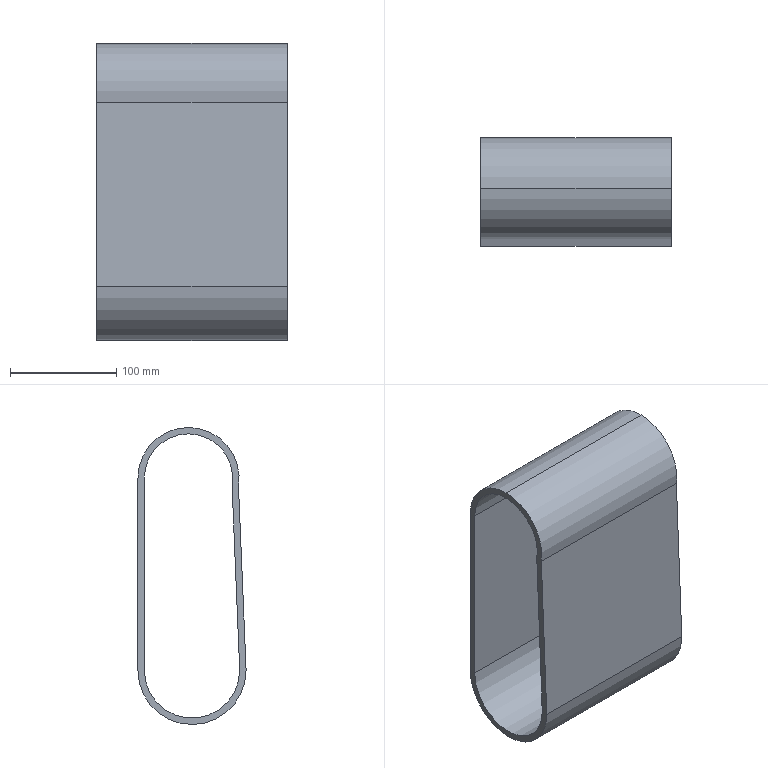Part | NX | 1 solid | 12 faces | box 180 x 102 x 280.001 mm | volume 706349 mm3 | cylinder 6 | plane 6 | commonest cylinder face diameters 83.424 x2 95.424 x2 90 x1 102 x1
STEP:
#1=CARTESIAN_POINT('',(220.674,202.789,606.798));
#2=VERTEX_POINT('',#1);
#3=CARTESIAN_POINT('',(220.674,244.501,565.086));
#4=VERTEX_POINT('',#3);
#5=CARTESIAN_POINT('',(220.674,202.789,565.086));
#6=DIRECTION('',(-1.,0.,0.));
#7=DIRECTION('',(0.,0.,1.));
#8=AXIS2_PLACEMENT_3D('',#5,#6,#7);
#9=CIRCLE('',#8,41.712);
#10=EDGE_CURVE('',#2,#4,#9,.T.);
#11=ORIENTED_EDGE('',*,*,#10,.F.);
#12=CARTESIAN_POINT('',(40.674,202.789,606.798));
#13=VERTEX_POINT('',#12);
#14=CARTESIAN_POINT('',(518.674,202.789,606.798));
#15=DIRECTION('',(-1.,0.,0.));
#16=VECTOR('',#15,1.);
#17=LINE('',#14,#16);
#18=EDGE_CURVE('',#2,#13,#17,.T.);
#19=ORIENTED_EDGE('',*,*,#18,.T.);
#20=CARTESIAN_POINT('',(40.674,244.501,565.086));
#21=VERTEX_POINT('',#20);
#22=CARTESIAN_POINT('',(40.674,202.789,565.086));
#23=DIRECTION('',(1.,0.,0.));
#24=DIRECTION('',(0.,0.,-1.));
#25=AXIS2_PLACEMENT_3D('',#22,#23,#24);
#26=CIRCLE('',#25,41.712);
#27=EDGE_CURVE('',#21,#13,#26,.T.);
#28=ORIENTED_EDGE('',*,*,#27,.F.);
#29=CARTESIAN_POINT('',(518.674,244.501,565.086));
#30=DIRECTION('',(-1.,0.,0.));
#31=VECTOR('',#30,1.);
#32=LINE('',#29,#31);
#33=EDGE_CURVE('',#4,#21,#32,.T.);
#34=ORIENTED_EDGE('',*,*,#33,.F.);
#35=EDGE_LOOP('',(#11,#19,#28,#34));
#36=FACE_OUTER_BOUND('',#35,.T.);
#37=CARTESIAN_POINT('',(518.674,202.789,565.086));
#38=DIRECTION('',(-1.,0.,0.));
#39=DIRECTION('',(0.,0.,1.));
#40=AXIS2_PLACEMENT_3D('',#37,#38,#39);
#41=CYLINDRICAL_SURFACE('',#40,41.712);
#42=ADVANCED_FACE('',(#36),#41,.F.);
#43=CARTESIAN_POINT('',(220.674,155.708,557.353));
#44=VERTEX_POINT('',#43);
#45=CARTESIAN_POINT('',(220.674,202.789,612.798));
#46=VERTEX_POINT('',#45);
#47=CARTESIAN_POINT('',(220.674,202.789,565.086));
#48=DIRECTION('',(-1.,0.,0.));
#49=DIRECTION('',(0.,0.,1.));
#50=AXIS2_PLACEMENT_3D('',#47,#48,#49);
#51=CIRCLE('',#50,47.712);
#52=EDGE_CURVE('',#44,#46,#51,.T.);
#53=ORIENTED_EDGE('',*,*,#52,.T.);
#54=CARTESIAN_POINT('',(40.674,202.789,612.798));
#55=VERTEX_POINT('',#54);
#56=CARTESIAN_POINT('',(518.674,202.789,612.798));
#57=DIRECTION('',(-1.,0.,0.));
#58=VECTOR('',#57,1.);
#59=LINE('',#56,#58);
#60=EDGE_CURVE('',#46,#55,#59,.T.);
#61=ORIENTED_EDGE('',*,*,#60,.T.);
#62=CARTESIAN_POINT('',(40.674,155.708,557.353));
#63=VERTEX_POINT('',#62);
#64=CARTESIAN_POINT('',(40.674,202.789,565.086));
#65=DIRECTION('',(1.,0.,0.));
#66=DIRECTION('',(0.,0.,-1.));
#67=AXIS2_PLACEMENT_3D('',#64,#65,#66);
#68=CIRCLE('',#67,47.712);
#69=EDGE_CURVE('',#55,#63,#68,.T.);
#70=ORIENTED_EDGE('',*,*,#69,.T.);
#71=CARTESIAN_POINT('',(518.674,155.708,557.353));
#72=DIRECTION('',(-1.,0.,0.));
#73=VECTOR('',#72,1.);
#74=LINE('',#71,#73);
#75=EDGE_CURVE('',#44,#63,#74,.T.);
#76=ORIENTED_EDGE('',*,*,#75,.F.);
#77=EDGE_LOOP('',(#53,#61,#70,#76));
#78=FACE_OUTER_BOUND('',#77,.T.);
#79=CARTESIAN_POINT('',(518.674,202.789,565.086));
#80=DIRECTION('',(-1.,0.,0.));
#81=DIRECTION('',(0.,0.,1.));
#82=AXIS2_PLACEMENT_3D('',#79,#80,#81);
#83=CYLINDRICAL_SURFACE('',#82,47.712);
#84=ADVANCED_FACE('',(#78),#83,.T.);
#85=CARTESIAN_POINT('',(40.674,148.501,383.926));
#86=VERTEX_POINT('',#85);
#87=CARTESIAN_POINT('',(40.674,250.501,383.798));
#88=VERTEX_POINT('',#87);
#89=CARTESIAN_POINT('',(40.674,199.501,383.798));
#90=DIRECTION('',(1.,0.,0.));
#91=DIRECTION('',(0.,0.,-1.));
#92=AXIS2_PLACEMENT_3D('',#89,#90,#91);
#93=CIRCLE('',#92,51.);
#94=EDGE_CURVE('',#86,#88,#93,.T.);
#95=ORIENTED_EDGE('',*,*,#94,.F.);
#96=CARTESIAN_POINT('',(40.674,148.506,384.047));
#97=DIRECTION('',(0.,-0.04152,-0.9991));
#98=VECTOR('',#97,1.);
#99=LINE('',#96,#98);
#100=EDGE_CURVE('',#63,#86,#99,.T.);
#101=ORIENTED_EDGE('',*,*,#100,.F.);
#102=ORIENTED_EDGE('',*,*,#69,.F.);
#103=CARTESIAN_POINT('',(40.674,250.501,565.086));
#104=VERTEX_POINT('',#103);
#105=CARTESIAN_POINT('',(40.674,202.789,565.086));
#106=DIRECTION('',(1.,0.,0.));
#107=DIRECTION('',(0.,0.,-1.));
#108=AXIS2_PLACEMENT_3D('',#105,#106,#107);
#109=CIRCLE('',#108,47.712);
#110=EDGE_CURVE('',#104,#55,#109,.T.);
#111=ORIENTED_EDGE('',*,*,#110,.F.);
#112=CARTESIAN_POINT('',(40.674,250.501,383.798));
#113=DIRECTION('',(0.,0.,1.));
#114=VECTOR('',#113,1.);
#115=LINE('',#112,#114);
#116=EDGE_CURVE('',#88,#104,#115,.T.);
#117=ORIENTED_EDGE('',*,*,#116,.F.);
#118=EDGE_LOOP('',(#95,#101,#102,#111,#117));
#119=FACE_BOUND('',#118,.T.);
#120=CARTESIAN_POINT('',(40.674,154.501,383.798));
#121=VERTEX_POINT('',#120);
#122=CARTESIAN_POINT('',(40.674,244.501,383.798));
#123=VERTEX_POINT('',#122);
#124=CARTESIAN_POINT('',(40.674,199.501,383.798));
#125=DIRECTION('',(1.,0.,0.));
#126=DIRECTION('',(0.,0.,-1.));
#127=AXIS2_PLACEMENT_3D('',#124,#125,#126);
#128=CIRCLE('',#127,45.);
#129=EDGE_CURVE('',#121,#123,#128,.T.);
#130=ORIENTED_EDGE('',*,*,#129,.T.);
#131=CARTESIAN_POINT('',(40.674,244.501,383.798));
#132=DIRECTION('',(0.,0.,1.));
#133=VECTOR('',#132,1.);
#134=LINE('',#131,#133);
#135=EDGE_CURVE('',#123,#21,#134,.T.);
#136=ORIENTED_EDGE('',*,*,#135,.T.);
#137=ORIENTED_EDGE('',*,*,#27,.T.);
#138=CARTESIAN_POINT('',(40.674,161.729,557.739));
#139=VERTEX_POINT('',#138);
#140=CARTESIAN_POINT('',(40.674,202.789,565.086));
#141=DIRECTION('',(1.,0.,0.));
#142=DIRECTION('',(0.,0.,-1.));
#143=AXIS2_PLACEMENT_3D('',#140,#141,#142);
#144=CIRCLE('',#143,41.712);
#145=EDGE_CURVE('',#13,#139,#144,.T.);
#146=ORIENTED_EDGE('',*,*,#145,.T.);
#147=CARTESIAN_POINT('',(40.674,154.501,383.798));
#148=DIRECTION('',(0.,-0.04152,-0.9991));
#149=VECTOR('',#148,1.);
#150=LINE('',#147,#149);
#151=EDGE_CURVE('',#139,#121,#150,.T.);
#152=ORIENTED_EDGE('',*,*,#151,.T.);
#153=EDGE_LOOP('',(#130,#136,#137,#146,#152));
#154=FACE_BOUND('',#153,.T.);
#155=CARTESIAN_POINT('',(40.674,199.501,383.798));
#156=DIRECTION('',(1.,0.,0.));
#157=DIRECTION('',(0.,0.,-1.));
#158=AXIS2_PLACEMENT_3D('',#155,#156,#157);
#159=PLANE('',#158);
#160=ADVANCED_FACE('',(#119,#154),#159,.F.);
#161=CARTESIAN_POINT('',(220.674,250.501,383.798));
#162=VERTEX_POINT('',#161);
#163=CARTESIAN_POINT('',(518.674,250.501,383.798));
#164=DIRECTION('',(-1.,0.,0.));
#165=VECTOR('',#164,1.);
#166=LINE('',#163,#165);
#167=EDGE_CURVE('',#162,#88,#166,.T.);
#168=ORIENTED_EDGE('',*,*,#167,.F.);
#169=CARTESIAN_POINT('',(220.674,148.501,383.926));
#170=VERTEX_POINT('',#169);
#171=CARTESIAN_POINT('',(220.674,199.501,383.798));
#172=DIRECTION('',(-1.,0.,0.));
#173=DIRECTION('',(0.,0.,1.));
#174=AXIS2_PLACEMENT_3D('',#171,#172,#173);
#175=CIRCLE('',#174,51.);
#176=EDGE_CURVE('',#162,#170,#175,.T.);
#177=ORIENTED_EDGE('',*,*,#176,.T.);
#178=CARTESIAN_POINT('',(518.674,148.501,383.926));
#179=DIRECTION('',(-1.,0.,0.));
#180=VECTOR('',#179,1.);
#181=LINE('',#178,#180);
#182=EDGE_CURVE('',#170,#86,#181,.T.);
#183=ORIENTED_EDGE('',*,*,#182,.T.);
#184=ORIENTED_EDGE('',*,*,#94,.T.);
#185=EDGE_LOOP('',(#168,#177,#183,#184));
#186=FACE_OUTER_BOUND('',#185,.T.);
#187=CARTESIAN_POINT('',(518.674,199.501,383.798));
#188=DIRECTION('',(-1.,0.,0.));
#189=DIRECTION('',(0.,0.,1.));
#190=AXIS2_PLACEMENT_3D('',#187,#188,#189);
#191=CYLINDRICAL_SURFACE('',#190,51.);
#192=ADVANCED_FACE('',(#186),#191,.T.);
#193=CARTESIAN_POINT('',(220.674,250.501,565.086));
#194=VERTEX_POINT('',#193);
#195=CARTESIAN_POINT('',(518.674,250.501,565.086));
#196=DIRECTION('',(-1.,0.,0.));
#197=VECTOR('',#196,1.);
#198=LINE('',#195,#197);
#199=EDGE_CURVE('',#194,#104,#198,.T.);
#200=ORIENTED_EDGE('',*,*,#199,.F.);
#201=CARTESIAN_POINT('',(220.674,250.501,383.798));
#202=DIRECTION('',(0.,0.,-1.));
#203=VECTOR('',#202,1.);
#204=LINE('',#201,#203);
#205=EDGE_CURVE('',#194,#162,#204,.T.);
#206=ORIENTED_EDGE('',*,*,#205,.T.);
#207=ORIENTED_EDGE('',*,*,#167,.T.);
#208=ORIENTED_EDGE('',*,*,#116,.T.);
#209=EDGE_LOOP('',(#200,#206,#207,#208));
#210=FACE_OUTER_BOUND('',#209,.T.);
#211=CARTESIAN_POINT('',(518.674,250.501,383.798));
#212=DIRECTION('',(0.,-1.,0.));
#213=DIRECTION('',(0.,0.,-1.));
#214=AXIS2_PLACEMENT_3D('',#211,#212,#213);
#215=PLANE('',#214);
#216=ADVANCED_FACE('',(#210),#215,.F.);
#217=ORIENTED_EDGE('',*,*,#60,.F.);
#218=CARTESIAN_POINT('',(220.674,202.789,565.086));
#219=DIRECTION('',(-1.,0.,0.));
#220=DIRECTION('',(0.,0.,1.));
#221=AXIS2_PLACEMENT_3D('',#218,#219,#220);
#222=CIRCLE('',#221,47.712);
#223=EDGE_CURVE('',#46,#194,#222,.T.);
#224=ORIENTED_EDGE('',*,*,#223,.T.);
#225=ORIENTED_EDGE('',*,*,#199,.T.);
#226=ORIENTED_EDGE('',*,*,#110,.T.);
#227=EDGE_LOOP('',(#217,#224,#225,#226));
#228=FACE_OUTER_BOUND('',#227,.T.);
#229=CARTESIAN_POINT('',(518.674,202.789,565.086));
#230=DIRECTION('',(-1.,0.,0.));
#231=DIRECTION('',(0.,0.,1.));
#232=AXIS2_PLACEMENT_3D('',#229,#230,#231);
#233=CYLINDRICAL_SURFACE('',#232,47.712);
#234=ADVANCED_FACE('',(#228),#233,.T.);
#235=ORIENTED_EDGE('',*,*,#182,.F.);
#236=CARTESIAN_POINT('',(220.674,148.506,384.047));
#237=DIRECTION('',(0.,0.04152,0.9991));
#238=VECTOR('',#237,1.);
#239=LINE('',#236,#238);
#240=EDGE_CURVE('',#170,#44,#239,.T.);
#241=ORIENTED_EDGE('',*,*,#240,.T.);
#242=ORIENTED_EDGE('',*,*,#75,.T.);
#243=ORIENTED_EDGE('',*,*,#100,.T.);
#244=EDGE_LOOP('',(#235,#241,#242,#243));
#245=FACE_OUTER_BOUND('',#244,.T.);
#246=CARTESIAN_POINT('',(518.674,148.506,384.047));
#247=DIRECTION('',(0.,0.9991,-0.04152));
#248=DIRECTION('',(0.,0.04152,0.9991));
#249=AXIS2_PLACEMENT_3D('',#246,#247,#248);
#250=PLANE('',#249);
#251=ADVANCED_FACE('',(#245),#250,.F.);
#252=CARTESIAN_POINT('',(220.674,244.501,383.798));
#253=VERTEX_POINT('',#252);
#254=CARTESIAN_POINT('',(220.674,154.501,383.798));
#255=VERTEX_POINT('',#254);
#256=CARTESIAN_POINT('',(220.674,199.501,383.798));
#257=DIRECTION('',(-1.,0.,0.));
#258=DIRECTION('',(0.,0.,1.));
#259=AXIS2_PLACEMENT_3D('',#256,#257,#258);
#260=CIRCLE('',#259,45.);
#261=EDGE_CURVE('',#253,#255,#260,.T.);
#262=ORIENTED_EDGE('',*,*,#261,.F.);
#263=CARTESIAN_POINT('',(518.674,244.501,383.798));
#264=DIRECTION('',(-1.,0.,0.));
#265=VECTOR('',#264,1.);
#266=LINE('',#263,#265);
#267=EDGE_CURVE('',#253,#123,#266,.T.);
#268=ORIENTED_EDGE('',*,*,#267,.T.);
#269=ORIENTED_EDGE('',*,*,#129,.F.);
#270=CARTESIAN_POINT('',(518.674,154.501,383.798));
#271=DIRECTION('',(-1.,0.,0.));
#272=VECTOR('',#271,1.);
#273=LINE('',#270,#272);
#274=EDGE_CURVE('',#255,#121,#273,.T.);
#275=ORIENTED_EDGE('',*,*,#274,.F.);
#276=EDGE_LOOP('',(#262,#268,#269,#275));
#277=FACE_OUTER_BOUND('',#276,.T.);
#278=CARTESIAN_POINT('',(518.674,199.501,383.798));
#279=DIRECTION('',(-1.,0.,0.));
#280=DIRECTION('',(0.,0.,1.));
#281=AXIS2_PLACEMENT_3D('',#278,#279,#280);
#282=CYLINDRICAL_SURFACE('',#281,45.);
#283=ADVANCED_FACE('',(#277),#282,.F.);
#284=CARTESIAN_POINT('',(220.674,244.501,383.798));
#285=DIRECTION('',(0.,0.,-1.));
#286=VECTOR('',#285,1.);
#287=LINE('',#284,#286);
#288=EDGE_CURVE('',#4,#253,#287,.T.);
#289=ORIENTED_EDGE('',*,*,#288,.F.);
#290=ORIENTED_EDGE('',*,*,#33,.T.);
#291=ORIENTED_EDGE('',*,*,#135,.F.);
#292=ORIENTED_EDGE('',*,*,#267,.F.);
#293=EDGE_LOOP('',(#289,#290,#291,#292));
#294=FACE_OUTER_BOUND('',#293,.T.);
#295=CARTESIAN_POINT('',(518.674,244.501,383.798));
#296=DIRECTION('',(0.,-1.,0.));
#297=DIRECTION('',(0.,0.,-1.));
#298=AXIS2_PLACEMENT_3D('',#295,#296,#297);
#299=PLANE('',#298);
#300=ADVANCED_FACE('',(#294),#299,.T.);
#301=ORIENTED_EDGE('',*,*,#18,.F.);
#302=CARTESIAN_POINT('',(220.674,161.729,557.739));
#303=VERTEX_POINT('',#302);
#304=CARTESIAN_POINT('',(220.674,202.789,565.086));
#305=DIRECTION('',(-1.,0.,0.));
#306=DIRECTION('',(0.,0.,1.));
#307=AXIS2_PLACEMENT_3D('',#304,#305,#306);
#308=CIRCLE('',#307,41.712);
#309=EDGE_CURVE('',#303,#2,#308,.T.);
#310=ORIENTED_EDGE('',*,*,#309,.F.);
#311=CARTESIAN_POINT('',(518.674,161.729,557.739));
#312=DIRECTION('',(-1.,0.,0.));
#313=VECTOR('',#312,1.);
#314=LINE('',#311,#313);
#315=EDGE_CURVE('',#303,#139,#314,.T.);
#316=ORIENTED_EDGE('',*,*,#315,.T.);
#317=ORIENTED_EDGE('',*,*,#145,.F.);
#318=EDGE_LOOP('',(#301,#310,#316,#317));
#319=FACE_OUTER_BOUND('',#318,.T.);
#320=CARTESIAN_POINT('',(518.674,202.789,565.086));
#321=DIRECTION('',(-1.,0.,0.));
#322=DIRECTION('',(0.,0.,1.));
#323=AXIS2_PLACEMENT_3D('',#320,#321,#322);
#324=CYLINDRICAL_SURFACE('',#323,41.712);
#325=ADVANCED_FACE('',(#319),#324,.F.);
#326=CARTESIAN_POINT('',(220.674,154.501,383.798));
#327=DIRECTION('',(0.,0.04152,0.9991));
#328=VECTOR('',#327,1.);
#329=LINE('',#326,#328);
#330=EDGE_CURVE('',#255,#303,#329,.T.);
#331=ORIENTED_EDGE('',*,*,#330,.F.);
#332=ORIENTED_EDGE('',*,*,#274,.T.);
#333=ORIENTED_EDGE('',*,*,#151,.F.);
#334=ORIENTED_EDGE('',*,*,#315,.F.);
#335=EDGE_LOOP('',(#331,#332,#333,#334));
#336=FACE_OUTER_BOUND('',#335,.T.);
#337=CARTESIAN_POINT('',(518.674,154.501,383.798));
#338=DIRECTION('',(0.,0.9991,-0.04152));
#339=DIRECTION('',(0.,0.04152,0.9991));
#340=AXIS2_PLACEMENT_3D('',#337,#338,#339);
#341=PLANE('',#340);
#342=ADVANCED_FACE('',(#336),#341,.T.);
#343=ORIENTED_EDGE('',*,*,#261,.T.);
#344=ORIENTED_EDGE('',*,*,#330,.T.);
#345=ORIENTED_EDGE('',*,*,#309,.T.);
#346=ORIENTED_EDGE('',*,*,#10,.T.);
#347=ORIENTED_EDGE('',*,*,#288,.T.);
#348=EDGE_LOOP('',(#343,#344,#345,#346,#347));
#349=FACE_BOUND('',#348,.T.);
#350=ORIENTED_EDGE('',*,*,#205,.F.);
#351=ORIENTED_EDGE('',*,*,#223,.F.);
#352=ORIENTED_EDGE('',*,*,#52,.F.);
#353=ORIENTED_EDGE('',*,*,#240,.F.);
#354=ORIENTED_EDGE('',*,*,#176,.F.);
#355=EDGE_LOOP('',(#350,#351,#352,#353,#354));
#356=FACE_BOUND('',#355,.T.);
#357=CARTESIAN_POINT('',(220.674,-484.499,2185.086));
#358=DIRECTION('',(-1.,0.,0.));
#359=DIRECTION('',(0.,0.,1.));
#360=AXIS2_PLACEMENT_3D('',#357,#358,#359);
#361=PLANE('',#360);
#362=ADVANCED_FACE('',(#349,#356),#361,.F.);
#363=CLOSED_SHELL('',(#42,#84,#160,#192,#216,#234,#251,#283,#300,#325,#342,#362));
#364=MANIFOLD_SOLID_BREP('',#363);
#365=(LENGTH_UNIT()NAMED_UNIT(*)SI_UNIT(.MILLI.,.METRE.));
#366=UNCERTAINTY_MEASURE_WITH_UNIT(LENGTH_MEASURE(0.00002),#365,'','');
#367=(NAMED_UNIT(*)PLANE_ANGLE_UNIT()SI_UNIT($,.RADIAN.));
#368=PLANE_ANGLE_MEASURE_WITH_UNIT(PLANE_ANGLE_MEASURE(0.01745),#367);
#369=DIMENSIONAL_EXPONENTS(0.,0.,0.,0.,0.,0.,0.);
#370=(CONVERSION_BASED_UNIT('DEGREE',#368)NAMED_UNIT(#369)PLANE_ANGLE_UNIT());
#371=(NAMED_UNIT(*)SI_UNIT($,.STERADIAN.)SOLID_ANGLE_UNIT());
#372=(GEOMETRIC_REPRESENTATION_CONTEXT(3)GLOBAL_UNCERTAINTY_ASSIGNED_CONTEXT((#366))GLOBAL_UNIT_ASSIGNED_CONTEXT((#365,#370,#371))REPRESENTATION_CONTEXT('',''));
#373=ADVANCED_BREP_SHAPE_REPRESENTATION('',(#364),#372);